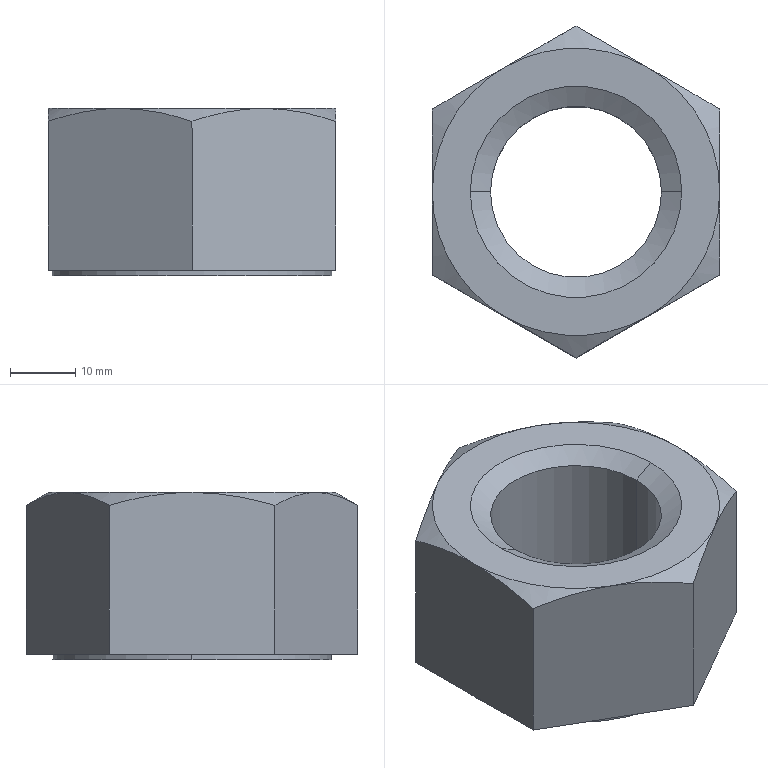Part | SolidWorks | features ICE 2, RevCut 2, Extrusion 1 | 1 solid | 23 faces | box 44.037 x 50.85 x 25.6 mm | volume 28405 mm3 | cone 10 | plane 9 | cylinder 4 | commonest cylinder face diameters 26.211 x2 42.8 x2
STEP:
#1=CARTESIAN_POINT('',(21.4,0.,-25.6));
#2=VERTEX_POINT('',#1);
#3=CARTESIAN_POINT('',(-21.4,0.,-25.6));
#4=VERTEX_POINT('',#3);
#5=CARTESIAN_POINT('',(0.,0.,-25.6));
#6=DIRECTION('',(0.,0.,1.));
#7=DIRECTION('',(1.,0.,0.));
#8=AXIS2_PLACEMENT_3D('',#5,#6,#7);
#9=CIRCLE('',#8,21.4);
#10=EDGE_CURVE('',#2,#4,#9,.T.);
#11=ORIENTED_EDGE('',*,*,#10,.T.);
#12=CARTESIAN_POINT('',(-21.4,0.,-24.8));
#13=VERTEX_POINT('',#12);
#14=CARTESIAN_POINT('',(-21.4,0.,0.));
#15=DIRECTION('',(0.,0.,1.));
#16=VECTOR('',#15,1000.);
#17=LINE('',#14,#16);
#18=EDGE_CURVE('',#4,#13,#17,.T.);
#19=ORIENTED_EDGE('',*,*,#18,.T.);
#20=CARTESIAN_POINT('',(21.4,0.,-24.8));
#21=VERTEX_POINT('',#20);
#22=CARTESIAN_POINT('',(0.,0.,-24.8));
#23=DIRECTION('',(0.,0.,1.));
#24=DIRECTION('',(1.,0.,0.));
#25=AXIS2_PLACEMENT_3D('',#22,#23,#24);
#26=CIRCLE('',#25,21.4);
#27=EDGE_CURVE('',#21,#13,#26,.T.);
#28=ORIENTED_EDGE('',*,*,#27,.F.);
#29=CARTESIAN_POINT('',(21.4,0.,0.));
#30=DIRECTION('',(0.,0.,1.));
#31=VECTOR('',#30,1000.);
#32=LINE('',#29,#31);
#33=EDGE_CURVE('',#2,#21,#32,.T.);
#34=ORIENTED_EDGE('',*,*,#33,.F.);
#35=EDGE_LOOP('',(#11,#19,#28,#34));
#36=FACE_OUTER_BOUND('',#35,.T.);
#37=CARTESIAN_POINT('',(0.,0.,0.));
#38=DIRECTION('',(0.,0.,1.));
#39=DIRECTION('',(1.,0.,0.));
#40=AXIS2_PLACEMENT_3D('',#37,#38,#39);
#41=CYLINDRICAL_SURFACE('',#40,21.4);
#42=ADVANCED_FACE('',(#36),#41,.T.);
#43=CARTESIAN_POINT('',(-13.106,0.,-23.813));
#44=VERTEX_POINT('',#43);
#45=CARTESIAN_POINT('',(13.106,0.,-23.813));
#46=VERTEX_POINT('',#45);
#47=CARTESIAN_POINT('',(0.,0.,-23.813));
#48=DIRECTION('',(0.,0.,1.));
#49=DIRECTION('',(1.,0.,0.));
#50=AXIS2_PLACEMENT_3D('',#47,#48,#49);
#51=CIRCLE('',#50,13.106);
#52=EDGE_CURVE('',#44,#46,#51,.T.);
#53=ORIENTED_EDGE('',*,*,#52,.T.);
#54=CARTESIAN_POINT('',(16.2,0.,-25.6));
#55=VERTEX_POINT('',#54);
#56=CARTESIAN_POINT('',(16.2,0.,-25.6));
#57=DIRECTION('',(0.866,0.,-0.5));
#58=VECTOR('',#57,1000.);
#59=LINE('',#56,#58);
#60=EDGE_CURVE('',#46,#55,#59,.T.);
#61=ORIENTED_EDGE('',*,*,#60,.T.);
#62=CARTESIAN_POINT('',(-16.2,0.,-25.6));
#63=VERTEX_POINT('',#62);
#64=CARTESIAN_POINT('',(0.,0.,-25.6));
#65=DIRECTION('',(0.,0.,1.));
#66=DIRECTION('',(1.,0.,0.));
#67=AXIS2_PLACEMENT_3D('',#64,#65,#66);
#68=CIRCLE('',#67,16.2);
#69=EDGE_CURVE('',#63,#55,#68,.T.);
#70=ORIENTED_EDGE('',*,*,#69,.F.);
#71=CARTESIAN_POINT('',(-16.2,0.,-25.6));
#72=DIRECTION('',(-0.866,0.,-0.5));
#73=VECTOR('',#72,1000.);
#74=LINE('',#71,#73);
#75=EDGE_CURVE('',#44,#63,#74,.T.);
#76=ORIENTED_EDGE('',*,*,#75,.F.);
#77=EDGE_LOOP('',(#53,#61,#70,#76));
#78=FACE_OUTER_BOUND('',#77,.T.);
#79=CARTESIAN_POINT('',(0.,0.,-25.6));
#80=DIRECTION('',(0.,0.,-1.));
#81=DIRECTION('',(-1.,0.,0.));
#82=AXIS2_PLACEMENT_3D('',#79,#80,#81);
#83=CONICAL_SURFACE('',#82,16.2,1.047);
#84=ADVANCED_FACE('',(#78),#83,.F.);
#85=CARTESIAN_POINT('',(-13.106,0.,-1.787));
#86=VERTEX_POINT('',#85);
#87=CARTESIAN_POINT('',(13.106,0.,-1.787));
#88=VERTEX_POINT('',#87);
#89=CARTESIAN_POINT('',(0.,0.,-1.787));
#90=DIRECTION('',(0.,0.,1.));
#91=DIRECTION('',(1.,0.,0.));
#92=AXIS2_PLACEMENT_3D('',#89,#90,#91);
#93=CIRCLE('',#92,13.106);
#94=EDGE_CURVE('',#86,#88,#93,.T.);
#95=ORIENTED_EDGE('',*,*,#94,.F.);
#96=CARTESIAN_POINT('',(-16.2,0.,0.));
#97=VERTEX_POINT('',#96);
#98=CARTESIAN_POINT('',(-13.106,0.,-1.787));
#99=DIRECTION('',(-0.866,0.,0.5));
#100=VECTOR('',#99,1000.);
#101=LINE('',#98,#100);
#102=EDGE_CURVE('',#86,#97,#101,.T.);
#103=ORIENTED_EDGE('',*,*,#102,.T.);
#104=CARTESIAN_POINT('',(16.2,0.,0.));
#105=VERTEX_POINT('',#104);
#106=CARTESIAN_POINT('',(0.,0.,0.));
#107=DIRECTION('',(0.,0.,1.));
#108=DIRECTION('',(1.,0.,0.));
#109=AXIS2_PLACEMENT_3D('',#106,#107,#108);
#110=CIRCLE('',#109,16.2);
#111=EDGE_CURVE('',#97,#105,#110,.T.);
#112=ORIENTED_EDGE('',*,*,#111,.T.);
#113=CARTESIAN_POINT('',(13.106,0.,-1.787));
#114=DIRECTION('',(0.866,0.,0.5));
#115=VECTOR('',#114,1000.);
#116=LINE('',#113,#115);
#117=EDGE_CURVE('',#88,#105,#116,.T.);
#118=ORIENTED_EDGE('',*,*,#117,.F.);
#119=EDGE_LOOP('',(#95,#103,#112,#118));
#120=FACE_OUTER_BOUND('',#119,.T.);
#121=CARTESIAN_POINT('',(0.,0.,-1.787));
#122=DIRECTION('',(0.,0.,1.));
#123=DIRECTION('',(1.,0.,0.));
#124=AXIS2_PLACEMENT_3D('',#121,#122,#123);
#125=CONICAL_SURFACE('',#124,13.106,1.047);
#126=ADVANCED_FACE('',(#120),#125,.F.);
#127=ORIENTED_EDGE('',*,*,#52,.F.);
#128=CARTESIAN_POINT('',(-13.106,0.,-25.6));
#129=DIRECTION('',(0.,0.,1.));
#130=VECTOR('',#129,1000.);
#131=LINE('',#128,#130);
#132=EDGE_CURVE('',#44,#86,#131,.T.);
#133=ORIENTED_EDGE('',*,*,#132,.T.);
#134=ORIENTED_EDGE('',*,*,#94,.T.);
#135=CARTESIAN_POINT('',(13.106,0.,-25.6));
#136=DIRECTION('',(0.,0.,1.));
#137=VECTOR('',#136,1000.);
#138=LINE('',#135,#137);
#139=EDGE_CURVE('',#46,#88,#138,.T.);
#140=ORIENTED_EDGE('',*,*,#139,.F.);
#141=EDGE_LOOP('',(#127,#133,#134,#140));
#142=FACE_OUTER_BOUND('',#141,.T.);
#143=CARTESIAN_POINT('',(0.,0.,-25.6));
#144=DIRECTION('',(0.,0.,1.));
#145=DIRECTION('',(1.,0.,0.));
#146=AXIS2_PLACEMENT_3D('',#143,#144,#145);
#147=CYLINDRICAL_SURFACE('',#146,13.106);
#148=ADVANCED_FACE('',(#142),#147,.F.);
#149=CARTESIAN_POINT('',(22.019,12.713,-24.8));
#150=VERTEX_POINT('',#149);
#151=CARTESIAN_POINT('',(22.019,12.713,-1.967));
#152=VERTEX_POINT('',#151);
#153=CARTESIAN_POINT('',(22.019,12.713,-25.6));
#154=DIRECTION('',(0.,0.,1.));
#155=VECTOR('',#154,1000.);
#156=LINE('',#153,#155);
#157=EDGE_CURVE('',#150,#152,#156,.T.);
#158=ORIENTED_EDGE('',*,*,#157,.F.);
#159=CARTESIAN_POINT('',(0.,25.425,-24.8));
#160=VERTEX_POINT('',#159);
#161=CARTESIAN_POINT('',(22.019,12.713,-24.8));
#162=DIRECTION('',(-0.866,0.5,0.));
#163=VECTOR('',#162,1000.);
#164=LINE('',#161,#163);
#165=EDGE_CURVE('',#150,#160,#164,.T.);
#166=ORIENTED_EDGE('',*,*,#165,.T.);
#167=CARTESIAN_POINT('',(0.,25.425,-1.967));
#168=VERTEX_POINT('',#167);
#169=CARTESIAN_POINT('',(0.,25.425,-25.6));
#170=DIRECTION('',(0.,0.,1.));
#171=VECTOR('',#170,1000.);
#172=LINE('',#169,#171);
#173=EDGE_CURVE('',#160,#168,#172,.T.);
#174=ORIENTED_EDGE('',*,*,#173,.T.);
#175=CARTESIAN_POINT('',(11.009,19.069,0.));
#176=VERTEX_POINT('',#175);
#177=CARTESIAN_POINT('',(0.,25.425,-1.967));
#178=CARTESIAN_POINT('',(1.801,24.385,-1.366));
#179=CARTESIAN_POINT('',(3.615,23.338,-0.8717));
#180=CARTESIAN_POINT('',(7.281,21.221,-0.1874));
#181=CARTESIAN_POINT('',(9.134,20.152,0.));
#182=CARTESIAN_POINT('',(11.009,19.069,0.));
#183=B_SPLINE_CURVE_WITH_KNOTS('',3,(#177,#178,#179,#180,#181,#182),.UNSPECIFIED.,.F.,.F.,(4,2,4),(0.000000238,0.006432,0.01286),.UNSPECIFIED.);
#184=EDGE_CURVE('',#168,#176,#183,.T.);
#185=ORIENTED_EDGE('',*,*,#184,.T.);
#186=CARTESIAN_POINT('',(11.009,19.069,0.));
#187=CARTESIAN_POINT('',(11.477,18.799,0.));
#188=CARTESIAN_POINT('',(11.946,18.528,-0.01153));
#189=CARTESIAN_POINT('',(12.881,17.988,-0.05729));
#190=CARTESIAN_POINT('',(13.346,17.719,-0.09146));
#191=CARTESIAN_POINT('',(14.739,16.916,-0.2264));
#192=CARTESIAN_POINT('',(15.661,16.383,-0.3596));
#193=CARTESIAN_POINT('',(18.411,14.796,-0.8735));
#194=CARTESIAN_POINT('',(20.222,13.75,-1.368));
#195=CARTESIAN_POINT('',(22.019,12.713,-1.967));
#196=B_SPLINE_CURVE_WITH_KNOTS('',3,(#186,#187,#188,#189,#190,#191,#192,#193,#194,#195),.UNSPECIFIED.,.F.,.F.,(4,2,2,2,4),(0.01286,0.01447,0.01607,0.01927,0.02568),.UNSPECIFIED.);
#197=EDGE_CURVE('',#176,#152,#196,.T.);
#198=ORIENTED_EDGE('',*,*,#197,.T.);
#199=EDGE_LOOP('',(#158,#166,#174,#185,#198));
#200=FACE_OUTER_BOUND('',#199,.T.);
#201=CARTESIAN_POINT('',(22.019,12.713,-25.6));
#202=DIRECTION('',(0.5,0.866,0.));
#203=DIRECTION('',(-0.866,0.5,0.));
#204=AXIS2_PLACEMENT_3D('',#201,#202,#203);
#205=PLANE('',#204);
#206=ADVANCED_FACE('',(#200),#205,.T.);
#207=CARTESIAN_POINT('',(22.019,-12.712,-24.8));
#208=VERTEX_POINT('',#207);
#209=CARTESIAN_POINT('',(22.019,-12.712,-1.967));
#210=VERTEX_POINT('',#209);
#211=CARTESIAN_POINT('',(22.019,-12.712,-25.6));
#212=DIRECTION('',(0.,0.,1.));
#213=VECTOR('',#212,1000.);
#214=LINE('',#211,#213);
#215=EDGE_CURVE('',#208,#210,#214,.T.);
#216=ORIENTED_EDGE('',*,*,#215,.F.);
#217=CARTESIAN_POINT('',(22.019,-12.712,-24.8));
#218=DIRECTION('',(0.,1.,0.));
#219=VECTOR('',#218,1000.);
#220=LINE('',#217,#219);
#221=EDGE_CURVE('',#208,#150,#220,.T.);
#222=ORIENTED_EDGE('',*,*,#221,.T.);
#223=ORIENTED_EDGE('',*,*,#157,.T.);
#224=CARTESIAN_POINT('',(22.019,0.,0.));
#225=VERTEX_POINT('',#224);
#226=CARTESIAN_POINT('',(22.019,12.713,-1.967));
#227=CARTESIAN_POINT('',(22.019,10.657,-1.373));
#228=CARTESIAN_POINT('',(22.019,8.574,-0.8791));
#229=CARTESIAN_POINT('',(22.019,5.391,-0.3623));
#230=CARTESIAN_POINT('',(22.019,4.32,-0.2276));
#231=CARTESIAN_POINT('',(22.019,2.155,-0.04574));
#232=CARTESIAN_POINT('',(22.019,1.075,0.));
#233=CARTESIAN_POINT('',(22.019,0.,0.));
#234=B_SPLINE_CURVE_WITH_KNOTS('',3,(#226,#227,#228,#229,#230,#231,#232,#233),.UNSPECIFIED.,.F.,.F.,(4,2,2,4),(0.05693,0.06337,0.06659,0.06981),.UNSPECIFIED.);
#235=EDGE_CURVE('',#152,#225,#234,.T.);
#236=ORIENTED_EDGE('',*,*,#235,.T.);
#237=CARTESIAN_POINT('',(22.019,0.,0.));
#238=CARTESIAN_POINT('',(22.019,-2.149,0.));
#239=CARTESIAN_POINT('',(22.019,-4.284,-0.1848));
#240=CARTESIAN_POINT('',(22.019,-7.466,-0.698));
#241=CARTESIAN_POINT('',(22.019,-8.523,-0.9078));
#242=CARTESIAN_POINT('',(22.019,-10.633,-1.394));
#243=CARTESIAN_POINT('',(22.019,-11.678,-1.668));
#244=CARTESIAN_POINT('',(22.019,-12.712,-1.967));
#245=B_SPLINE_CURVE_WITH_KNOTS('',3,(#237,#238,#239,#240,#241,#242,#243,#244),.UNSPECIFIED.,.F.,.F.,(4,2,2,4),(0.06981,0.07625,0.07947,0.08269),.UNSPECIFIED.);
#246=EDGE_CURVE('',#225,#210,#245,.T.);
#247=ORIENTED_EDGE('',*,*,#246,.T.);
#248=EDGE_LOOP('',(#216,#222,#223,#236,#247));
#249=FACE_OUTER_BOUND('',#248,.T.);
#250=CARTESIAN_POINT('',(22.019,-12.712,-25.6));
#251=DIRECTION('',(1.,0.,0.));
#252=DIRECTION('',(0.,1.,0.));
#253=AXIS2_PLACEMENT_3D('',#250,#251,#252);
#254=PLANE('',#253);
#255=ADVANCED_FACE('',(#249),#254,.T.);
#256=CARTESIAN_POINT('',(0.,-25.425,-24.8));
#257=VERTEX_POINT('',#256);
#258=CARTESIAN_POINT('',(0.,-25.425,-1.967));
#259=VERTEX_POINT('',#258);
#260=CARTESIAN_POINT('',(0.,-25.425,-25.6));
#261=DIRECTION('',(0.,0.,1.));
#262=VECTOR('',#261,1000.);
#263=LINE('',#260,#262);
#264=EDGE_CURVE('',#257,#259,#263,.T.);
#265=ORIENTED_EDGE('',*,*,#264,.F.);
#266=CARTESIAN_POINT('',(0.,-25.425,-24.8));
#267=DIRECTION('',(0.866,0.5,0.));
#268=VECTOR('',#267,1000.);
#269=LINE('',#266,#268);
#270=EDGE_CURVE('',#257,#208,#269,.T.);
#271=ORIENTED_EDGE('',*,*,#270,.T.);
#272=ORIENTED_EDGE('',*,*,#215,.T.);
#273=CARTESIAN_POINT('',(11.009,-19.069,0.));
#274=VERTEX_POINT('',#273);
#275=CARTESIAN_POINT('',(22.019,-12.712,-1.967));
#276=CARTESIAN_POINT('',(20.218,-13.752,-1.366));
#277=CARTESIAN_POINT('',(18.404,-14.8,-0.8717));
#278=CARTESIAN_POINT('',(14.737,-16.916,-0.1874));
#279=CARTESIAN_POINT('',(12.885,-17.986,0.));
#280=CARTESIAN_POINT('',(11.009,-19.069,0.));
#281=B_SPLINE_CURVE_WITH_KNOTS('',3,(#275,#276,#277,#278,#279,#280),.UNSPECIFIED.,.F.,.F.,(4,2,4),(0.000000238,0.006432,0.01286),.UNSPECIFIED.);
#282=EDGE_CURVE('',#210,#274,#281,.T.);
#283=ORIENTED_EDGE('',*,*,#282,.T.);
#284=CARTESIAN_POINT('',(11.009,-19.069,0.));
#285=CARTESIAN_POINT('',(10.542,-19.338,0.));
#286=CARTESIAN_POINT('',(10.073,-19.61,-0.01153));
#287=CARTESIAN_POINT('',(9.138,-20.149,-0.05729));
#288=CARTESIAN_POINT('',(8.672,-20.418,-0.09146));
#289=CARTESIAN_POINT('',(7.28,-21.222,-0.2264));
#290=CARTESIAN_POINT('',(6.358,-21.754,-0.3596));
#291=CARTESIAN_POINT('',(3.608,-23.342,-0.8735));
#292=CARTESIAN_POINT('',(1.796,-24.388,-1.368));
#293=CARTESIAN_POINT('',(0.,-25.425,-1.967));
#294=B_SPLINE_CURVE_WITH_KNOTS('',3,(#284,#285,#286,#287,#288,#289,#290,#291,#292,#293),.UNSPECIFIED.,.F.,.F.,(4,2,2,2,4),(0.01286,0.01447,0.01607,0.01927,0.02568),.UNSPECIFIED.);
#295=EDGE_CURVE('',#274,#259,#294,.T.);
#296=ORIENTED_EDGE('',*,*,#295,.T.);
#297=EDGE_LOOP('',(#265,#271,#272,#283,#296));
#298=FACE_OUTER_BOUND('',#297,.T.);
#299=CARTESIAN_POINT('',(0.,-25.425,-25.6));
#300=DIRECTION('',(0.5,-0.866,0.));
#301=DIRECTION('',(0.866,0.5,0.));
#302=AXIS2_PLACEMENT_3D('',#299,#300,#301);
#303=PLANE('',#302);
#304=ADVANCED_FACE('',(#298),#303,.T.);
#305=CARTESIAN_POINT('',(-22.019,-12.713,-24.8));
#306=VERTEX_POINT('',#305);
#307=CARTESIAN_POINT('',(-22.019,-12.712,-1.967));
#308=VERTEX_POINT('',#307);
#309=CARTESIAN_POINT('',(-22.019,-12.712,-25.6));
#310=DIRECTION('',(0.,0.,1.));
#311=VECTOR('',#310,1000.);
#312=LINE('',#309,#311);
#313=EDGE_CURVE('',#306,#308,#312,.T.);
#314=ORIENTED_EDGE('',*,*,#313,.F.);
#315=CARTESIAN_POINT('',(-22.019,-12.712,-24.8));
#316=DIRECTION('',(0.866,-0.5,0.));
#317=VECTOR('',#316,1000.);
#318=LINE('',#315,#317);
#319=EDGE_CURVE('',#306,#257,#318,.T.);
#320=ORIENTED_EDGE('',*,*,#319,.T.);
#321=ORIENTED_EDGE('',*,*,#264,.T.);
#322=CARTESIAN_POINT('',(-11.009,-19.069,0.));
#323=VERTEX_POINT('',#322);
#324=CARTESIAN_POINT('',(0.,-25.425,-1.967));
#325=CARTESIAN_POINT('',(-1.801,-24.385,-1.366));
#326=CARTESIAN_POINT('',(-3.615,-23.338,-0.8717));
#327=CARTESIAN_POINT('',(-7.281,-21.221,-0.1874));
#328=CARTESIAN_POINT('',(-9.134,-20.152,0.));
#329=CARTESIAN_POINT('',(-11.009,-19.069,0.));
#330=B_SPLINE_CURVE_WITH_KNOTS('',3,(#324,#325,#326,#327,#328,#329),.UNSPECIFIED.,.F.,.F.,(4,2,4),(0.000000238,0.006432,0.01286),.UNSPECIFIED.);
#331=EDGE_CURVE('',#259,#323,#330,.T.);
#332=ORIENTED_EDGE('',*,*,#331,.T.);
#333=CARTESIAN_POINT('',(-11.009,-19.069,0.));
#334=CARTESIAN_POINT('',(-11.477,-18.799,0.));
#335=CARTESIAN_POINT('',(-11.946,-18.528,-0.01153));
#336=CARTESIAN_POINT('',(-12.881,-17.988,-0.05729));
#337=CARTESIAN_POINT('',(-13.346,-17.719,-0.09146));
#338=CARTESIAN_POINT('',(-14.739,-16.916,-0.2264));
#339=CARTESIAN_POINT('',(-15.661,-16.383,-0.3596));
#340=CARTESIAN_POINT('',(-18.411,-14.796,-0.8735));
#341=CARTESIAN_POINT('',(-20.222,-13.75,-1.368));
#342=CARTESIAN_POINT('',(-22.019,-12.712,-1.967));
#343=B_SPLINE_CURVE_WITH_KNOTS('',3,(#333,#334,#335,#336,#337,#338,#339,#340,#341,#342),.UNSPECIFIED.,.F.,.F.,(4,2,2,2,4),(0.01286,0.01447,0.01607,0.01927,0.02568),.UNSPECIFIED.);
#344=EDGE_CURVE('',#323,#308,#343,.T.);
#345=ORIENTED_EDGE('',*,*,#344,.T.);
#346=EDGE_LOOP('',(#314,#320,#321,#332,#345));
#347=FACE_OUTER_BOUND('',#346,.T.);
#348=CARTESIAN_POINT('',(-22.019,-12.712,-25.6));
#349=DIRECTION('',(-0.5,-0.866,0.));
#350=DIRECTION('',(0.866,-0.5,0.));
#351=AXIS2_PLACEMENT_3D('',#348,#349,#350);
#352=PLANE('',#351);
#353=ADVANCED_FACE('',(#347),#352,.T.);
#354=CARTESIAN_POINT('',(-22.019,12.713,-24.8));
#355=VERTEX_POINT('',#354);
#356=CARTESIAN_POINT('',(-22.019,12.713,-1.967));
#357=VERTEX_POINT('',#356);
#358=CARTESIAN_POINT('',(-22.019,12.713,-25.6));
#359=DIRECTION('',(0.,0.,1.));
#360=VECTOR('',#359,1000.);
#361=LINE('',#358,#360);
#362=EDGE_CURVE('',#355,#357,#361,.T.);
#363=ORIENTED_EDGE('',*,*,#362,.F.);
#364=CARTESIAN_POINT('',(-22.019,12.713,-24.8));
#365=DIRECTION('',(0.,-1.,0.));
#366=VECTOR('',#365,1000.);
#367=LINE('',#364,#366);
#368=EDGE_CURVE('',#355,#306,#367,.T.);
#369=ORIENTED_EDGE('',*,*,#368,.T.);
#370=ORIENTED_EDGE('',*,*,#313,.T.);
#371=CARTESIAN_POINT('',(-22.019,0.,0.));
#372=VERTEX_POINT('',#371);
#373=CARTESIAN_POINT('',(-22.019,-12.712,-1.967));
#374=CARTESIAN_POINT('',(-22.019,-11.678,-1.668));
#375=CARTESIAN_POINT('',(-22.019,-10.633,-1.394));
#376=CARTESIAN_POINT('',(-22.019,-8.523,-0.9078));
#377=CARTESIAN_POINT('',(-22.019,-7.466,-0.698));
#378=CARTESIAN_POINT('',(-22.019,-4.284,-0.1848));
#379=CARTESIAN_POINT('',(-22.019,-2.149,0.));
#380=CARTESIAN_POINT('',(-22.019,0.,0.));
#381=B_SPLINE_CURVE_WITH_KNOTS('',3,(#373,#374,#375,#376,#377,#378,#379,#380),.UNSPECIFIED.,.F.,.F.,(4,2,2,4),(0.0231,0.02631,0.02953,0.03596),.UNSPECIFIED.);
#382=EDGE_CURVE('',#308,#372,#381,.T.);
#383=ORIENTED_EDGE('',*,*,#382,.T.);
#384=CARTESIAN_POINT('',(-22.019,0.,0.));
#385=CARTESIAN_POINT('',(-22.019,1.075,0.));
#386=CARTESIAN_POINT('',(-22.019,2.155,-0.04574));
#387=CARTESIAN_POINT('',(-22.019,4.32,-0.2276));
#388=CARTESIAN_POINT('',(-22.019,5.391,-0.3623));
#389=CARTESIAN_POINT('',(-22.019,8.574,-0.8791));
#390=CARTESIAN_POINT('',(-22.019,10.657,-1.373));
#391=CARTESIAN_POINT('',(-22.019,12.713,-1.967));
#392=B_SPLINE_CURVE_WITH_KNOTS('',3,(#384,#385,#386,#387,#388,#389,#390,#391),.UNSPECIFIED.,.F.,.F.,(4,2,2,4),(0.03596,0.03918,0.0424,0.04883),.UNSPECIFIED.);
#393=EDGE_CURVE('',#372,#357,#392,.T.);
#394=ORIENTED_EDGE('',*,*,#393,.T.);
#395=EDGE_LOOP('',(#363,#369,#370,#383,#394));
#396=FACE_OUTER_BOUND('',#395,.T.);
#397=CARTESIAN_POINT('',(-22.019,12.713,-25.6));
#398=DIRECTION('',(-1.,0.,0.));
#399=DIRECTION('',(0.,-1.,0.));
#400=AXIS2_PLACEMENT_3D('',#397,#398,#399);
#401=PLANE('',#400);
#402=ADVANCED_FACE('',(#396),#401,.T.);
#403=ORIENTED_EDGE('',*,*,#173,.F.);
#404=CARTESIAN_POINT('',(0.,25.425,-24.8));
#405=DIRECTION('',(-0.866,-0.5,0.));
#406=VECTOR('',#405,1000.);
#407=LINE('',#404,#406);
#408=EDGE_CURVE('',#160,#355,#407,.T.);
#409=ORIENTED_EDGE('',*,*,#408,.T.);
#410=ORIENTED_EDGE('',*,*,#362,.T.);
#411=CARTESIAN_POINT('',(-11.009,19.069,0.));
#412=VERTEX_POINT('',#411);
#413=CARTESIAN_POINT('',(-22.019,12.713,-1.967));
#414=CARTESIAN_POINT('',(-20.218,13.752,-1.366));
#415=CARTESIAN_POINT('',(-18.404,14.8,-0.8717));
#416=CARTESIAN_POINT('',(-14.737,16.916,-0.1874));
#417=CARTESIAN_POINT('',(-12.885,17.986,0.));
#418=CARTESIAN_POINT('',(-11.009,19.069,0.));
#419=B_SPLINE_CURVE_WITH_KNOTS('',3,(#413,#414,#415,#416,#417,#418),.UNSPECIFIED.,.F.,.F.,(4,2,4),(0.000000238,0.006432,0.01286),.UNSPECIFIED.);
#420=EDGE_CURVE('',#357,#412,#419,.T.);
#421=ORIENTED_EDGE('',*,*,#420,.T.);
#422=CARTESIAN_POINT('',(-11.009,19.069,0.));
#423=CARTESIAN_POINT('',(-10.542,19.338,0.));
#424=CARTESIAN_POINT('',(-10.073,19.61,-0.01153));
#425=CARTESIAN_POINT('',(-9.138,20.149,-0.05729));
#426=CARTESIAN_POINT('',(-8.672,20.418,-0.09146));
#427=CARTESIAN_POINT('',(-7.28,21.222,-0.2264));
#428=CARTESIAN_POINT('',(-6.358,21.754,-0.3596));
#429=CARTESIAN_POINT('',(-3.608,23.342,-0.8735));
#430=CARTESIAN_POINT('',(-1.796,24.388,-1.368));
#431=CARTESIAN_POINT('',(0.,25.425,-1.967));
#432=B_SPLINE_CURVE_WITH_KNOTS('',3,(#422,#423,#424,#425,#426,#427,#428,#429,#430,#431),.UNSPECIFIED.,.F.,.F.,(4,2,2,2,4),(0.01286,0.01447,0.01607,0.01927,0.02568),.UNSPECIFIED.);
#433=EDGE_CURVE('',#412,#168,#432,.T.);
#434=ORIENTED_EDGE('',*,*,#433,.T.);
#435=EDGE_LOOP('',(#403,#409,#410,#421,#434));
#436=FACE_OUTER_BOUND('',#435,.T.);
#437=CARTESIAN_POINT('',(0.,25.425,-25.6));
#438=DIRECTION('',(-0.5,0.866,0.));
#439=DIRECTION('',(-0.866,-0.5,0.));
#440=AXIS2_PLACEMENT_3D('',#437,#438,#439);
#441=PLANE('',#440);
#442=ADVANCED_FACE('',(#436),#441,.T.);
#443=ORIENTED_EDGE('',*,*,#69,.T.);
#444=CARTESIAN_POINT('',(0.,0.,-25.6));
#445=DIRECTION('',(0.,0.,1.));
#446=DIRECTION('',(1.,0.,0.));
#447=AXIS2_PLACEMENT_3D('',#444,#445,#446);
#448=CIRCLE('',#447,16.2);
#449=EDGE_CURVE('',#55,#63,#448,.T.);
#450=ORIENTED_EDGE('',*,*,#449,.T.);
#451=EDGE_LOOP('',(#443,#450));
#452=FACE_BOUND('',#451,.T.);
#453=ORIENTED_EDGE('',*,*,#10,.F.);
#454=CARTESIAN_POINT('',(0.,0.,-25.6));
#455=DIRECTION('',(0.,0.,1.));
#456=DIRECTION('',(1.,0.,0.));
#457=AXIS2_PLACEMENT_3D('',#454,#455,#456);
#458=CIRCLE('',#457,21.4);
#459=EDGE_CURVE('',#4,#2,#458,.T.);
#460=ORIENTED_EDGE('',*,*,#459,.F.);
#461=EDGE_LOOP('',(#453,#460));
#462=FACE_OUTER_BOUND('',#461,.T.);
#463=CARTESIAN_POINT('',(0.,25.425,-25.6));
#464=DIRECTION('',(0.,0.,1.));
#465=DIRECTION('',(1.,0.,0.));
#466=AXIS2_PLACEMENT_3D('',#463,#464,#465);
#467=PLANE('',#466);
#468=ADVANCED_FACE('',(#452,#462),#467,.F.);
#469=CARTESIAN_POINT('',(0.,0.,0.));
#470=DIRECTION('',(0.,0.,1.));
#471=DIRECTION('',(1.,0.,0.));
#472=AXIS2_PLACEMENT_3D('',#469,#470,#471);
#473=CIRCLE('',#472,16.2);
#474=EDGE_CURVE('',#105,#97,#473,.T.);
#475=ORIENTED_EDGE('',*,*,#474,.F.);
#476=ORIENTED_EDGE('',*,*,#111,.F.);
#477=EDGE_LOOP('',(#475,#476));
#478=FACE_BOUND('',#477,.T.);
#479=CARTESIAN_POINT('',(0.,0.,0.));
#480=DIRECTION('',(0.,0.,1.));
#481=DIRECTION('',(1.,0.,0.));
#482=AXIS2_PLACEMENT_3D('',#479,#480,#481);
#483=CIRCLE('',#482,22.019);
#484=EDGE_CURVE('',#274,#225,#483,.T.);
#485=ORIENTED_EDGE('',*,*,#484,.T.);
#486=CARTESIAN_POINT('',(0.,0.,0.));
#487=DIRECTION('',(0.,0.,1.));
#488=DIRECTION('',(1.,0.,0.));
#489=AXIS2_PLACEMENT_3D('',#486,#487,#488);
#490=CIRCLE('',#489,22.019);
#491=EDGE_CURVE('',#225,#176,#490,.T.);
#492=ORIENTED_EDGE('',*,*,#491,.T.);
#493=CARTESIAN_POINT('',(0.,0.,0.));
#494=DIRECTION('',(0.,0.,1.));
#495=DIRECTION('',(1.,0.,0.));
#496=AXIS2_PLACEMENT_3D('',#493,#494,#495);
#497=CIRCLE('',#496,22.019);
#498=EDGE_CURVE('',#176,#412,#497,.T.);
#499=ORIENTED_EDGE('',*,*,#498,.T.);
#500=CARTESIAN_POINT('',(0.,0.,0.));
#501=DIRECTION('',(0.,0.,1.));
#502=DIRECTION('',(1.,0.,0.));
#503=AXIS2_PLACEMENT_3D('',#500,#501,#502);
#504=CIRCLE('',#503,22.019);
#505=EDGE_CURVE('',#412,#372,#504,.T.);
#506=ORIENTED_EDGE('',*,*,#505,.T.);
#507=CARTESIAN_POINT('',(0.,0.,0.));
#508=DIRECTION('',(0.,0.,1.));
#509=DIRECTION('',(1.,0.,0.));
#510=AXIS2_PLACEMENT_3D('',#507,#508,#509);
#511=CIRCLE('',#510,22.019);
#512=EDGE_CURVE('',#372,#323,#511,.T.);
#513=ORIENTED_EDGE('',*,*,#512,.T.);
#514=CARTESIAN_POINT('',(0.,0.,0.));
#515=DIRECTION('',(0.,0.,1.));
#516=DIRECTION('',(1.,0.,0.));
#517=AXIS2_PLACEMENT_3D('',#514,#515,#516);
#518=CIRCLE('',#517,22.019);
#519=EDGE_CURVE('',#323,#274,#518,.T.);
#520=ORIENTED_EDGE('',*,*,#519,.T.);
#521=EDGE_LOOP('',(#485,#492,#499,#506,#513,#520));
#522=FACE_OUTER_BOUND('',#521,.T.);
#523=CARTESIAN_POINT('',(0.,25.425,0.));
#524=DIRECTION('',(0.,0.,1.));
#525=DIRECTION('',(1.,0.,0.));
#526=AXIS2_PLACEMENT_3D('',#523,#524,#525);
#527=PLANE('',#526);
#528=ADVANCED_FACE('',(#478,#522),#527,.T.);
#529=ORIENTED_EDGE('',*,*,#132,.F.);
#530=CARTESIAN_POINT('',(0.,0.,-23.813));
#531=DIRECTION('',(0.,0.,1.));
#532=DIRECTION('',(1.,0.,0.));
#533=AXIS2_PLACEMENT_3D('',#530,#531,#532);
#534=CIRCLE('',#533,13.106);
#535=EDGE_CURVE('',#46,#44,#534,.T.);
#536=ORIENTED_EDGE('',*,*,#535,.F.);
#537=ORIENTED_EDGE('',*,*,#139,.T.);
#538=CARTESIAN_POINT('',(0.,0.,-1.787));
#539=DIRECTION('',(0.,0.,1.));
#540=DIRECTION('',(1.,0.,0.));
#541=AXIS2_PLACEMENT_3D('',#538,#539,#540);
#542=CIRCLE('',#541,13.106);
#543=EDGE_CURVE('',#88,#86,#542,.T.);
#544=ORIENTED_EDGE('',*,*,#543,.T.);
#545=EDGE_LOOP('',(#529,#536,#537,#544));
#546=FACE_OUTER_BOUND('',#545,.T.);
#547=CARTESIAN_POINT('',(0.,0.,-25.6));
#548=DIRECTION('',(0.,0.,1.));
#549=DIRECTION('',(1.,0.,0.));
#550=AXIS2_PLACEMENT_3D('',#547,#548,#549);
#551=CYLINDRICAL_SURFACE('',#550,13.106);
#552=ADVANCED_FACE('',(#546),#551,.F.);
#553=ORIENTED_EDGE('',*,*,#102,.F.);
#554=ORIENTED_EDGE('',*,*,#543,.F.);
#555=ORIENTED_EDGE('',*,*,#117,.T.);
#556=ORIENTED_EDGE('',*,*,#474,.T.);
#557=EDGE_LOOP('',(#553,#554,#555,#556));
#558=FACE_OUTER_BOUND('',#557,.T.);
#559=CARTESIAN_POINT('',(0.,0.,-1.787));
#560=DIRECTION('',(0.,0.,1.));
#561=DIRECTION('',(1.,0.,0.));
#562=AXIS2_PLACEMENT_3D('',#559,#560,#561);
#563=CONICAL_SURFACE('',#562,13.106,1.047);
#564=ADVANCED_FACE('',(#558),#563,.F.);
#565=ORIENTED_EDGE('',*,*,#60,.F.);
#566=ORIENTED_EDGE('',*,*,#535,.T.);
#567=ORIENTED_EDGE('',*,*,#75,.T.);
#568=ORIENTED_EDGE('',*,*,#449,.F.);
#569=EDGE_LOOP('',(#565,#566,#567,#568));
#570=FACE_OUTER_BOUND('',#569,.T.);
#571=CARTESIAN_POINT('',(0.,0.,-25.6));
#572=DIRECTION('',(0.,0.,-1.));
#573=DIRECTION('',(-1.,0.,0.));
#574=AXIS2_PLACEMENT_3D('',#571,#572,#573);
#575=CONICAL_SURFACE('',#574,16.2,1.047);
#576=ADVANCED_FACE('',(#570),#575,.F.);
#577=ORIENTED_EDGE('',*,*,#433,.F.);
#578=ORIENTED_EDGE('',*,*,#498,.F.);
#579=ORIENTED_EDGE('',*,*,#184,.F.);
#580=EDGE_LOOP('',(#577,#578,#579));
#581=FACE_OUTER_BOUND('',#580,.T.);
#582=CARTESIAN_POINT('',(0.,0.,0.));
#583=DIRECTION('',(0.,0.,-1.));
#584=DIRECTION('',(1.,0.,0.));
#585=AXIS2_PLACEMENT_3D('',#582,#583,#584);
#586=CONICAL_SURFACE('',#585,22.019,1.047);
#587=ADVANCED_FACE('',(#581),#586,.T.);
#588=ORIENTED_EDGE('',*,*,#505,.F.);
#589=ORIENTED_EDGE('',*,*,#420,.F.);
#590=ORIENTED_EDGE('',*,*,#393,.F.);
#591=EDGE_LOOP('',(#588,#589,#590));
#592=FACE_OUTER_BOUND('',#591,.T.);
#593=CARTESIAN_POINT('',(0.,0.,0.));
#594=DIRECTION('',(0.,0.,-1.));
#595=DIRECTION('',(1.,0.,0.));
#596=AXIS2_PLACEMENT_3D('',#593,#594,#595);
#597=CONICAL_SURFACE('',#596,22.019,1.047);
#598=ADVANCED_FACE('',(#592),#597,.T.);
#599=ORIENTED_EDGE('',*,*,#512,.F.);
#600=ORIENTED_EDGE('',*,*,#382,.F.);
#601=ORIENTED_EDGE('',*,*,#344,.F.);
#602=EDGE_LOOP('',(#599,#600,#601));
#603=FACE_OUTER_BOUND('',#602,.T.);
#604=CARTESIAN_POINT('',(0.,0.,0.));
#605=DIRECTION('',(0.,0.,-1.));
#606=DIRECTION('',(1.,0.,0.));
#607=AXIS2_PLACEMENT_3D('',#604,#605,#606);
#608=CONICAL_SURFACE('',#607,22.019,1.047);
#609=ADVANCED_FACE('',(#603),#608,.T.);
#610=ORIENTED_EDGE('',*,*,#519,.F.);
#611=ORIENTED_EDGE('',*,*,#331,.F.);
#612=ORIENTED_EDGE('',*,*,#295,.F.);
#613=EDGE_LOOP('',(#610,#611,#612));
#614=FACE_OUTER_BOUND('',#613,.T.);
#615=CARTESIAN_POINT('',(0.,0.,0.));
#616=DIRECTION('',(0.,0.,-1.));
#617=DIRECTION('',(1.,0.,0.));
#618=AXIS2_PLACEMENT_3D('',#615,#616,#617);
#619=CONICAL_SURFACE('',#618,22.019,1.047);
#620=ADVANCED_FACE('',(#614),#619,.T.);
#621=ORIENTED_EDGE('',*,*,#484,.F.);
#622=ORIENTED_EDGE('',*,*,#282,.F.);
#623=ORIENTED_EDGE('',*,*,#246,.F.);
#624=EDGE_LOOP('',(#621,#622,#623));
#625=FACE_OUTER_BOUND('',#624,.T.);
#626=CARTESIAN_POINT('',(0.,0.,0.));
#627=DIRECTION('',(0.,0.,-1.));
#628=DIRECTION('',(1.,0.,0.));
#629=AXIS2_PLACEMENT_3D('',#626,#627,#628);
#630=CONICAL_SURFACE('',#629,22.019,1.047);
#631=ADVANCED_FACE('',(#625),#630,.T.);
#632=ORIENTED_EDGE('',*,*,#491,.F.);
#633=ORIENTED_EDGE('',*,*,#235,.F.);
#634=ORIENTED_EDGE('',*,*,#197,.F.);
#635=EDGE_LOOP('',(#632,#633,#634));
#636=FACE_OUTER_BOUND('',#635,.T.);
#637=CARTESIAN_POINT('',(0.,0.,0.));
#638=DIRECTION('',(0.,0.,-1.));
#639=DIRECTION('',(1.,0.,0.));
#640=AXIS2_PLACEMENT_3D('',#637,#638,#639);
#641=CONICAL_SURFACE('',#640,22.019,1.047);
#642=ADVANCED_FACE('',(#636),#641,.T.);
#643=ORIENTED_EDGE('',*,*,#18,.F.);
#644=ORIENTED_EDGE('',*,*,#459,.T.);
#645=ORIENTED_EDGE('',*,*,#33,.T.);
#646=CARTESIAN_POINT('',(0.,0.,-24.8));
#647=DIRECTION('',(0.,0.,1.));
#648=DIRECTION('',(1.,0.,0.));
#649=AXIS2_PLACEMENT_3D('',#646,#647,#648);
#650=CIRCLE('',#649,21.4);
#651=EDGE_CURVE('',#13,#21,#650,.T.);
#652=ORIENTED_EDGE('',*,*,#651,.F.);
#653=EDGE_LOOP('',(#643,#644,#645,#652));
#654=FACE_OUTER_BOUND('',#653,.T.);
#655=CARTESIAN_POINT('',(0.,0.,0.));
#656=DIRECTION('',(0.,0.,1.));
#657=DIRECTION('',(1.,0.,0.));
#658=AXIS2_PLACEMENT_3D('',#655,#656,#657);
#659=CYLINDRICAL_SURFACE('',#658,21.4);
#660=ADVANCED_FACE('',(#654),#659,.T.);
#661=ORIENTED_EDGE('',*,*,#27,.T.);
#662=ORIENTED_EDGE('',*,*,#651,.T.);
#663=EDGE_LOOP('',(#661,#662));
#664=FACE_BOUND('',#663,.T.);
#665=ORIENTED_EDGE('',*,*,#221,.F.);
#666=ORIENTED_EDGE('',*,*,#270,.F.);
#667=ORIENTED_EDGE('',*,*,#319,.F.);
#668=ORIENTED_EDGE('',*,*,#368,.F.);
#669=ORIENTED_EDGE('',*,*,#408,.F.);
#670=ORIENTED_EDGE('',*,*,#165,.F.);
#671=EDGE_LOOP('',(#665,#666,#667,#668,#669,#670));
#672=FACE_OUTER_BOUND('',#671,.T.);
#673=CARTESIAN_POINT('',(0.,-21.4,-24.8));
#674=DIRECTION('',(0.,0.,-1.));
#675=DIRECTION('',(-1.,0.,0.));
#676=AXIS2_PLACEMENT_3D('',#673,#674,#675);
#677=PLANE('',#676);
#678=ADVANCED_FACE('',(#664,#672),#677,.T.);
#679=CLOSED_SHELL('',(#42,#84,#126,#148,#206,#255,#304,#353,#402,#442,#468,#528,#552,#564,#576,#587,#598,#609,#620,#631,#642,#660,#678));
#680=MANIFOLD_SOLID_BREP('',#679);
#681=CARTESIAN_POINT('',(0.,0.,0.));
#682=DIRECTION('',(0.,0.,1.));
#683=DIRECTION('',(1.,0.,0.));
#684=AXIS2_PLACEMENT_3D('',#681,#682,#683);
#685=(LENGTH_UNIT()NAMED_UNIT(*)SI_UNIT(.MILLI.,.METRE.));
#686=UNCERTAINTY_MEASURE_WITH_UNIT(LENGTH_MEASURE(0.00001),#685,'','');
#687=(NAMED_UNIT(*)PLANE_ANGLE_UNIT()SI_UNIT($,.RADIAN.));
#688=(NAMED_UNIT(*)SI_UNIT($,.STERADIAN.)SOLID_ANGLE_UNIT());
#689=(GEOMETRIC_REPRESENTATION_CONTEXT(3)GLOBAL_UNCERTAINTY_ASSIGNED_CONTEXT((#686))GLOBAL_UNIT_ASSIGNED_CONTEXT((#685,#687,#688))REPRESENTATION_CONTEXT('',''));
#690=ADVANCED_BREP_SHAPE_REPRESENTATION('',(#680,#684),#689);